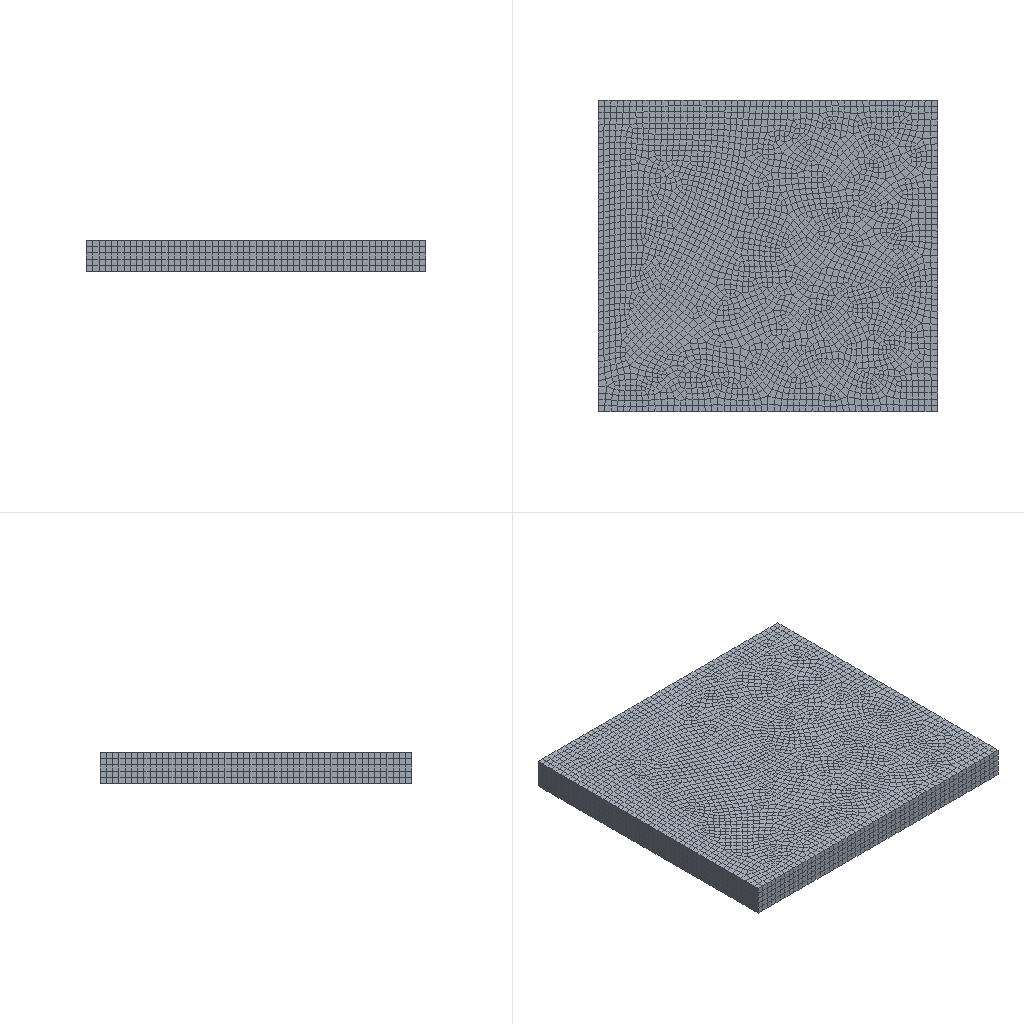Simulation study | abaqus
Set-up summary:
category,name,step,type,value,unit,region
solver,abaqus
solver,version,,,Abaqus/Explicit 2020
units,not stated in the deck,,not stated
analysis,deck,,transient,transient
load_step,Step-1,Step-1,transient
load_step,requested,,,1
mesh,nodes,,,20397
mesh,elements,,,16455
element_type,C3D8R,,solid,16220
element_type,COH3D8,,cohesive,235
load,load commands in deck,,count,1
bc,support commands in deck,,count,1
material,COH,,in results
material,MATERIAL-1,,in results
check,setup vs results,,match,"per instance, exact: element labels, types and connectivity; labels of the nodes the elements use; coordinates of those nodes at SINGLE_PRECISION in 1 of 1 instance(s)"
Abaqus input file, long lists of numbers shortened:
*Heading
** Job name: Job-1 Model name: Model-1
** Generated by: Abaqus/CAE 2020
*Preprint, echo=NO, model=NO, history=NO, contact=NO
**
** PARTS
**
*Part, name=Part-1
*Node
      1,   247.86,  -2112.528,           0.
      2,           0.,  -2184.625,           0.
** (20395 more lines like these left out)
*Element, type=C3D8R
   1,   652,   564,    22,    21,  7828,  7740,  2714,  2713
   2,   656,   655, 20270, 20268,  7832,  7831, 20269, 20267
** (16218 more lines like these left out)
*Element, type=COH3D8
16221,   109,  2613,   150,     6, 20098, 20097, 20096, 20095
16222,  2614,  2613,   109,   110, 20100, 20097, 20098, 20099
** (233 more lines like these left out)
*Nset, nset=Set-5, generate
     1,  20376,      1
*Elset, elset=Set-5, generate
     1,  16220,      1
*Elset, elset=CohesiveSeam-1-Elements, generate
 16221,  16455,      1
*Nset, nset=CohesiveSeam-1-TopNodes
     1,     9,   158,   159,   160,   161, 20095, 20096, 20097, 20098, 20099, 20100, 20101, 20102, 20103, 20104
 20105, 20106, 20107, 20108, 20109, 20110, 20111, 20112, 20113, 20114, 20115, 20116, 20117, 20118, 20119, 20120
** (16 more lines like these left out)
*Nset, nset=CohesiveSeam-1-BottomNodes
    1,    4,    5,    6,    7,    9,   10,   11,   12,   13,   91,   92,   93,   94,   95,   96
   97,   98,   99,  100,  101,  102,  103,  104,  105,  106,  107,  108,  109,  110,  111,  112
** (16 more lines like these left out)
*Nset, nset=CohesiveSeam-1-MidNodes
   1,   9, 158, 159, 160, 161
*Elset, elset=__PickedSurf6_S2, internal, generate
 16221,  16455,      1
*Elset, elset=__PickedSurf6_S5, internal, generate
  4940,  14244,   2326
*Elset, elset=__PickedSurf6_S4, internal
  4941,  4944,  5409,  7267,  7270,  7735,  9593,  9596, 10061, 11919, 11922, 12387, 14245, 14248, 14713
*Elset, elset=__PickedSurf6_S6, internal, generate
  5410,  14714,   2326
*Surface, type=ELEMENT, name=_PickedSurf6, internal
__PickedSurf6_S2, S2
__PickedSurf6_S5, S5
__PickedSurf6_S4, S4
__PickedSurf6_S6, S6
*Elset, elset=__PickedSurf14_S2, internal, generate
 16221,  16455,      1
*Surface, type=ELEMENT, name=_PickedSurf14, internal
__PickedSurf14_S2, S2
*Elset, elset=_CohesiveSeam-1-TopSurf_S2, internal, generate
 16221,  16455,      1
*Surface, type=ELEMENT, name=CohesiveSeam-1-TopSurf
_CohesiveSeam-1-TopSurf_S2, S2
*Elset, elset=_CohesiveSeam-1-BottomSurf_S1, internal, generate
 16221,  16455,      1
*Surface, type=ELEMENT, name=CohesiveSeam-1-BottomSurf
_CohesiveSeam-1-BottomSurf_S1, S1
** Section: Section-1
*Solid Section, elset=Set-5, material=Material-1
,
** Section: coh
*Cohesive Section, elset=CohesiveSeam-1-Elements, controls=EC-1, material=coh, response=TRACTION SEPARATION
,
*End Part
**
**
** ASSEMBLY
**
*Assembly, name=Assembly
**
*Instance, name=Part-1-1, part=Part-1
*End Instance
**
*Nset, nset=Set-2, instance=Part-1-1
   15,   16,   19,   20,  280,  281,  282,  283,  284,  285,  286,  287,  288,  289,  290,  291
  292,  293,  294,  295,  296,  297,  298,  299,  300,  301,  302,  303,  304,  305,  306,  307
** (19 more lines like these left out)
*Elset, elset=Set-2, instance=Part-1-1
  4592,  4594,  4595,  4596,  4598,  4618,  4629,  4630,  4703,  4713,  4714,  4718,  4720,  4743,  4755,  4766
  4772,  4773,  4805,  4806,  4823,  5099,  5104,  5105,  5411,  5420,  5536,  5537,  5539,  5541,  5542,  5544
** (15 more lines like these left out)
*Elset, elset=_Surf-1_S3, internal, instance=Part-1-1
    5,   11,   48,   52,   53,   55,   56,   65,  117,  159,  923,  929,  966,  970,  971,  973
  974,  983, 1035, 1077, 1841, 1847, 1884, 1888, 1889, 1891, 1892, 1901, 1953, 1995, 2759, 2765
** (2 more lines like these left out)
*Elset, elset=_Surf-1_S5, internal, instance=Part-1-1
    9,   50,   51,   57,   60,   62,   66,  115,  116,  121,  149,  162,  168,  927,  968,  969
  975,  978,  980,  984, 1033, 1034, 1039, 1067, 1080, 1086, 1845, 1886, 1887, 1893, 1896, 1898
** (3 more lines like these left out)
*Elset, elset=_Surf-1_S6, internal, instance=Part-1-1, generate
   47,  3719,   918
*Surface, type=ELEMENT, name=Surf-1
_Surf-1_S3, S3
_Surf-1_S5, S5
_Surf-1_S6, S6
*End Assembly
**
** ELEMENT CONTROLS
**
*Section Controls, name=EC-1, ELEMENT DELETION=YES
1., 1., 1.
*Amplitude, name=Amp-1
             0.,              0.,            0.02,              1.
**
** MATERIALS
**
*Material, name=Material-1
*Density
 1.8e-09,
*Elastic
1550., 0.2
*Material, name=coh
*Damage Initiation, criterion=MAXS
5.,5.,5.
*Damage Evolution, type=DISPLACEMENT
 1e-11,
*Density
 1.8e-09,
*Elastic, type=TRACTION
1550.,1550.,1550.
**
** INTERACTION PROPERTIES
**
*Surface Interaction, name=IntProp-1
*Friction
 0.4,
*Surface Behavior, pressure-overclosure=HARD
** ----------------------------------------------------------------
**
** STEP: Step-1
**
*Step, name=Step-1, nlgeom=YES
*Dynamic, Explicit
, 0.1
*Bulk Viscosity
0.06, 1.2
** Mass Scaling: Semi-Automatic
**               Whole Model
*Fixed Mass Scaling, factor=50.
**
** BOUNDARY CONDITIONS
**
** Name: BC-1 Type: 对称/反对称/完全固定
*Boundary
Set-2, ENCASTRE
**
** LOADS
**
** Name: Load-1   Type: Pressure
*Dsload, amplitude=Amp-1
Surf-1, P, 10.
**
** INTERACTIONS
**
** Interaction: Int-1
*Contact, op=NEW
*Contact Inclusions, ALL EXTERIOR
*Contact Property Assignment
 ,  , IntProp-1
**
** OUTPUT REQUESTS
**
*Restart, write, number interval=1, time marks=NO
**
** FIELD OUTPUT: F-Output-1
**
*Output, field, number interval=50
*Node Output
A, CF, RF, RM, RT, U, V
*Element Output, directions=YES
E, EVF, LE, MISES, MISESMAX, PE, PEEQ, PEEQVAVG, PEVAVG, S, SDEG, SF, STATUS, SVAVG
*Contact Output
CDISP, CSTRESS
**
** HISTORY OUTPUT: H-Output-1
**
*Output, history, variable=PRESELECT
*End Step
Results summary:
result,step,Step-1,completed,increments=2384 time=0.1/0.1
result,analysis,,,transient
result,last_loadstep,,,1
result,primary field,,,U
result,reaction total,,FX,-439907.912,model units
result,reaction total,,FY,3322221.429,model units
result,reaction total,,FZ,-2350.665,model units